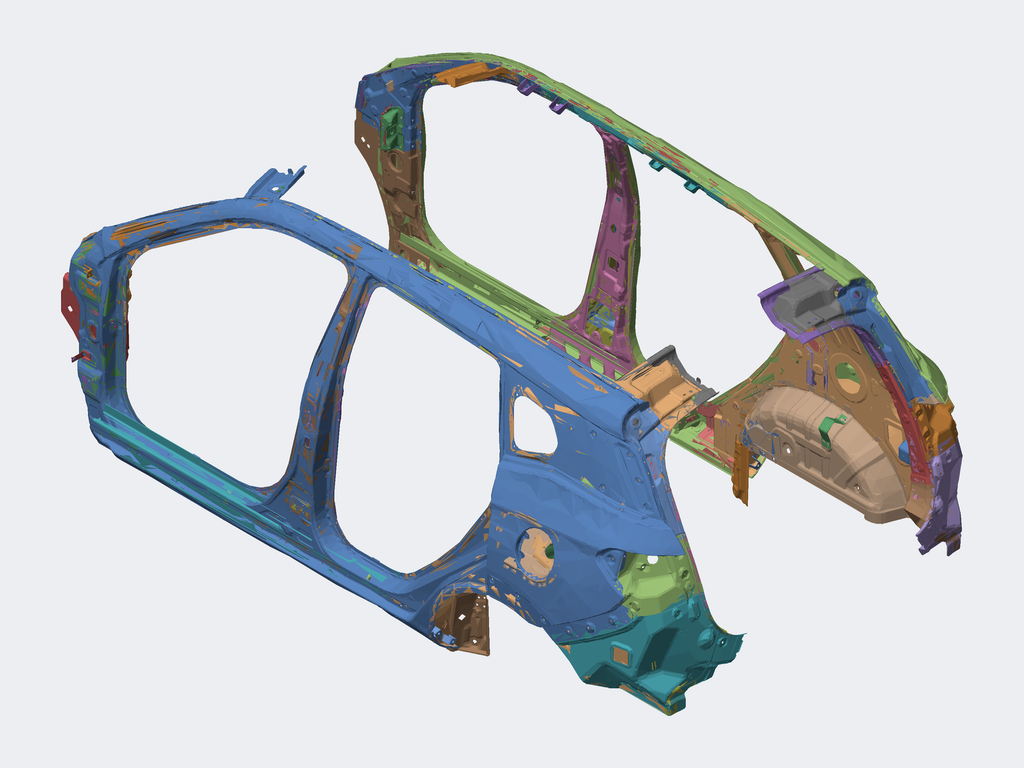Assembly | STEP file | 146 different items | 273 placed
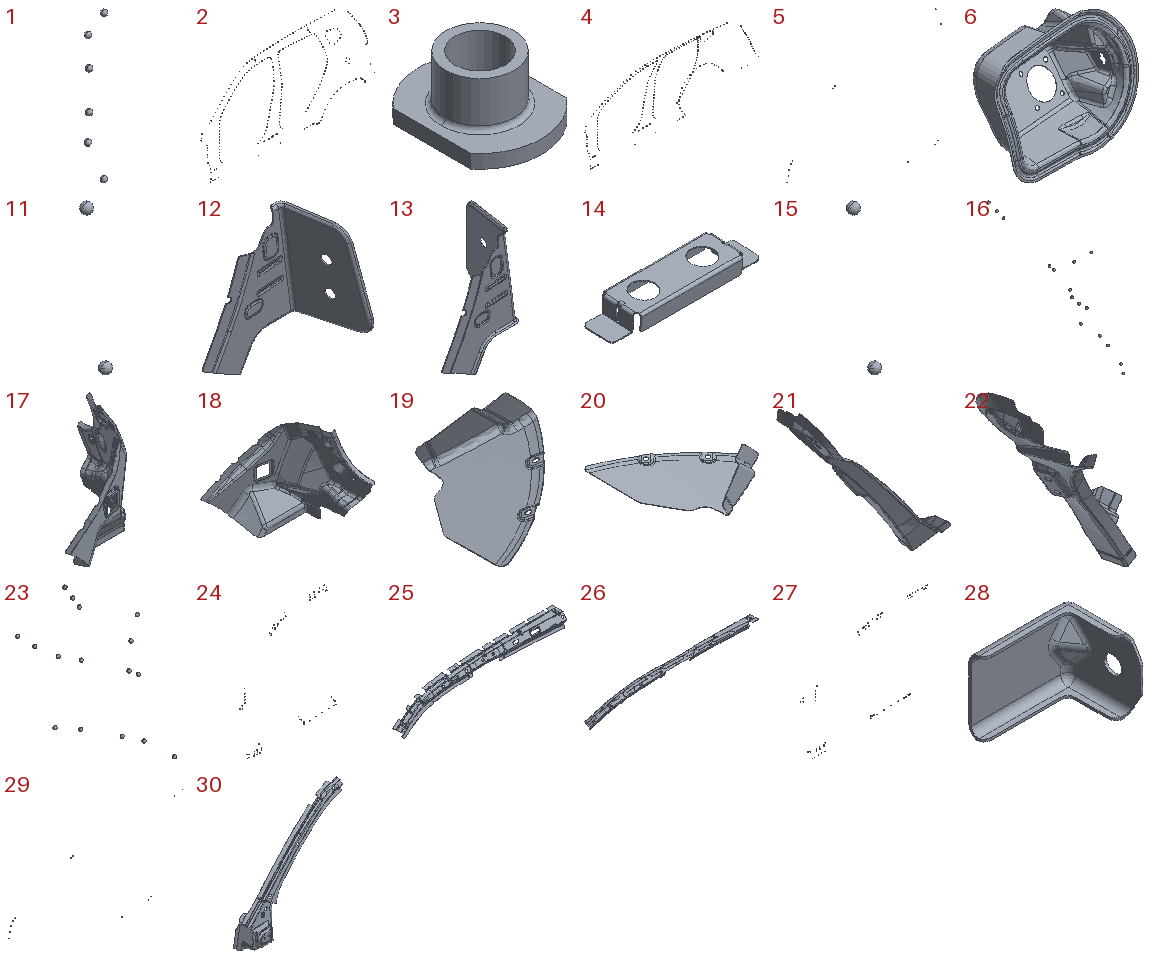Parts list (item | name | quantity | parent item | size | volume):
1 | FN5401370-H | x1 | in FNA5401370 | - | -
2 | FNA5401010-H | x1 | in FNA5401010 | - | -
3 | FNA5401011 | x12 | in FNA5401510, FNA5401520, FNA5401530, FNA5401540, FNA5401830, FNA5401840, FNA5401950, FNA5401960 | 21 x 27 x 13 mm | 2051 mm3
4 | FNA5401020-H | x1 | in FNA5401020 | - | -
5 | FNA5401100-H | x1 | in FNA5401100 | - | -
6 | FNA5401101 | x1 | in FNA5401110 | 305.711 x 153.486 x 230.44 mm | 76829 mm3
7 | FNA5401110-H | x1 | in FNA5401110 | - | -
8 | FNA5401111 | x1 | in FNA5401110 | - | -
9 | FNA5401112 | x1 | in FNA5401120 | - | -
10 | FNA5401120-H | x1 | in FNA5401120 | - | -
11 | FNA5401130-H | x1 | in FNA5401130 | - | -
12 | FNA5401131 | x1 | in FNA5401130 | 126.55 x 90.381 x 162.439 mm | 23457 mm3
13 | FNA5401132 | x1 | in FNA5401140 | 126.55 x 90.381 x 162.439 mm | 23442 mm3
14 | FNA5401133 | x4 | in FNA5401130, FNA5401140, FNA5401250, FNA5401260 | 102.073 x 26.855 x 12.87 mm | 2645 mm3
15 | FNA5401140-H | x1 | in FNA5401140 | - | -
16 | FNA5401150-H | x1 | in FNA5401150 | - | -
17 | FNA5401151 | x1 | in FNA5401150 | 516 x 448.464 x 475.039 mm | 197748 mm3
18 | FNA5401152 | x1 | in FNA5401160 | 516.001 x 448.464 x 475.039 mm | 197648 mm3
19 | FNA5401153 | x1 | in FNA5401150 | 165.89 x 168.782 x 61.393 mm | 13779 mm3
20 | FNA5401154 | x1 | in FNA5401160 | 165.89 x 168.782 x 61.393 mm | 13774 mm3
21 | FNA5401155 | x1 | in FNA5401150 | 332 x 187.997 x 427.512 mm | 56977 mm3
22 | FNA5401156 | x1 | in FNA5401160 | 332 x 187.997 x 427.512 mm | 56978 mm3
23 | FNA5401160-H | x1 | in FNA5401160 | - | -
24 | FNA5401170-H | x1 | in FNA5401170 | - | -
25 | FNA5401171 | x1 | in FNA5401170 | 1257 x 126.52 x 207.673 mm | 214669 mm3
26 | FNA5401172 | x1 | in FNA5401180 | 1257 x 126.52 x 207.673 mm | 214644 mm3
27 | FNA5401180-H | x1 | in FNA5401180 | - | -
28 | FNA5401191 | x2 | in FNA5401190 | 40.165 x 30.291 x 30.011 mm | 2314 mm3
29 | FNA5401200-H | x1 | in FNA5401200 | - | -
30 | FNA5401211 | x1 | in FNA5401210 | 914.927 x 216.551 x 677.274 mm | 215697 mm3
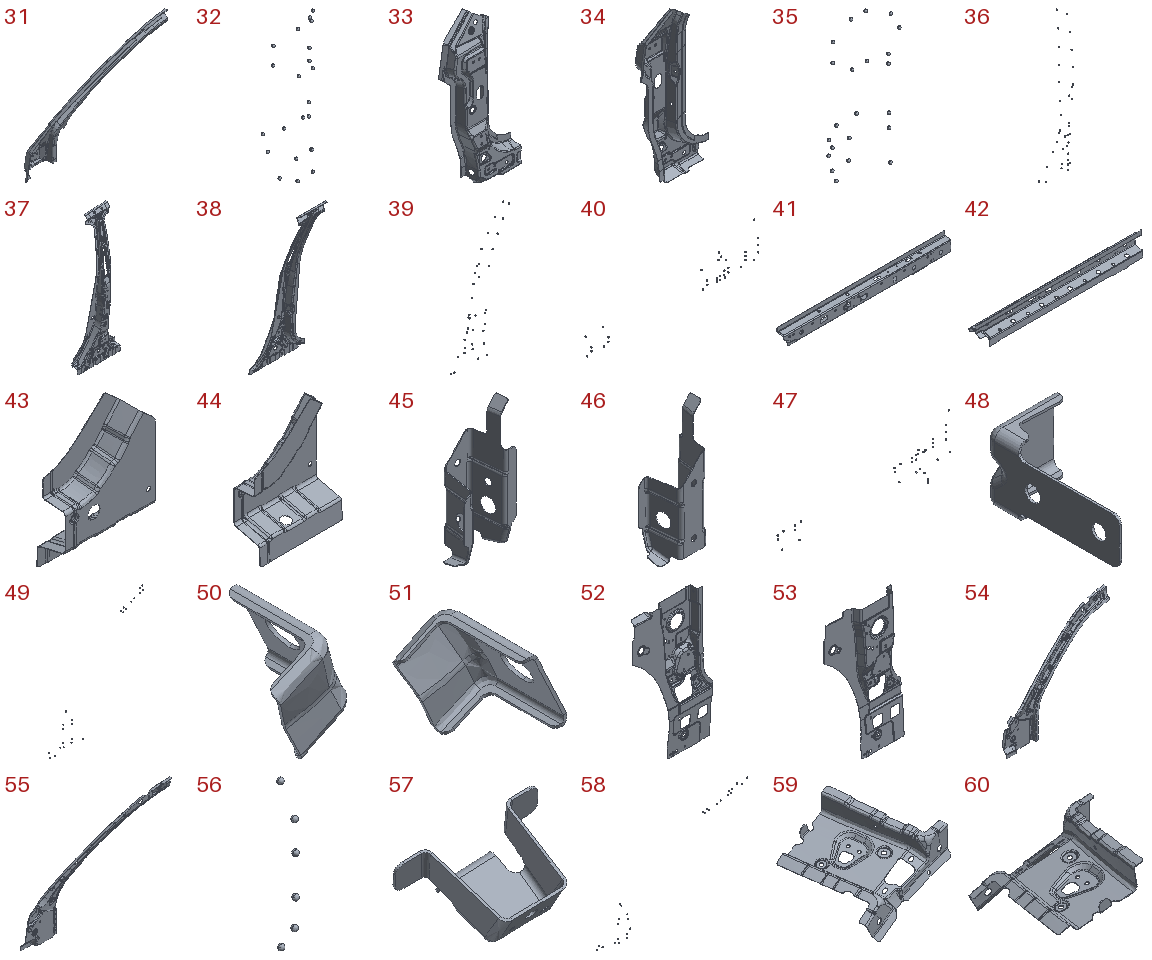31 | FNA5401212 | x1 | in FNA5401220 | 914.927 x 216.551 x 677.274 mm | 214602 mm3
32 | FNA5401230-H | x1 | in FNA5401230 | - | -
33 | FNA5401231 | x1 | in FNA5401230 | 393.159 x 114.364 x 853.043 mm | 316427 mm3
34 | FNA5401232 | x1 | in FNA5401240 | 393.159 x 114.364 x 853.043 mm | 316443 mm3
35 | FNA5401240-H | x1 | in FNA5401240 | - | -
36 | FNA5401250-H | x1 | in FNA5401250 | - | -
37 | FNA5401251 | x1 | in FNA5401250 | 510.856 x 226.55 x 1230 mm | 703654 mm3
38 | FNA5401252 | x1 | in FNA5401260 | 510.856 x 226.55 x 1230 mm | 703226 mm3
39 | FNA5401260-H | x1 | in FNA5401260 | - | -
40 | FNA5401270-H | x1 | in FNA5401270 | - | -
41 | FNA5401271 | x1 | in FNA5401270 | 1459 x 72.45 x 212.137 mm | 599256 mm3
42 | FNA5401272 | x1 | in FNA5401280 | 1459 x 72.45 x 212.137 mm | 599256 mm3
43 | FNA5401273 | x1 | in FNA5401270 | 220.5 x 72.73 x 306.154 mm | 92619 mm3
44 | FNA5401274 | x1 | in FNA5401280 | 220.5 x 72.73 x 306.154 mm | 92619 mm3
45 | FNA5401275 | x1 | in FNA5401270 | 90 x 57.5 x 220.985 mm | 30019 mm3
46 | FNA5401276 | x1 | in FNA5401280 | 90 x 57.5 x 220.985 mm | 30013 mm3
47 | FNA5401280-H | x1 | in FNA5401280 | - | -
48 | FNA5401291 | x2 | in FNA5401290 | 30.161 x 60.798 x 30.791 mm | 2443 mm3
49 | FNA5401300-H | x1 | in FNA5401300 | - | -
50 | FNA5401311 | x1 | in FNA5401300 | 33.614 x 36.273 x 38.59 mm | 2270 mm3
51 | FNA5401321 | x1 | in FNA5401400 | 33.613 x 36.273 x 38.59 mm | 2270 mm3
52 | FNA5401331 | x1 | in FNA5401330 | 367 x 39.355 x 636.857 mm | 124897 mm3
53 | FNA5401332 | x1 | in FNA5401340 | 367 x 39.355 x 636.857 mm | 124786 mm3
54 | FNA5401351 | x1 | in FNA5401350 | 1045 x 172.359 x 753.685 mm | 232138 mm3
55 | FNA5401352 | x1 | in FNA5401360 | 1045 x 172.359 x 753.685 mm | 232159 mm3
56 | FNA5401380-H | x1 | in FNA5401380 | - | -
57 | FNA5401391 | x2 | in FNA5401390 | 86.183 x 71.891 x 52.032 mm | 9472 mm3
58 | FNA5401400-H | x1 | in FNA5401400 | - | -
59 | FNA5401411 | x1 | in FNA5401410 | 243.972 x 240.219 x 155.739 mm | 51999 mm3
60 | FNA5401412 | x1 | in FNA5401420 | 243.972 x 240.219 x 155.739 mm | 52004 mm3
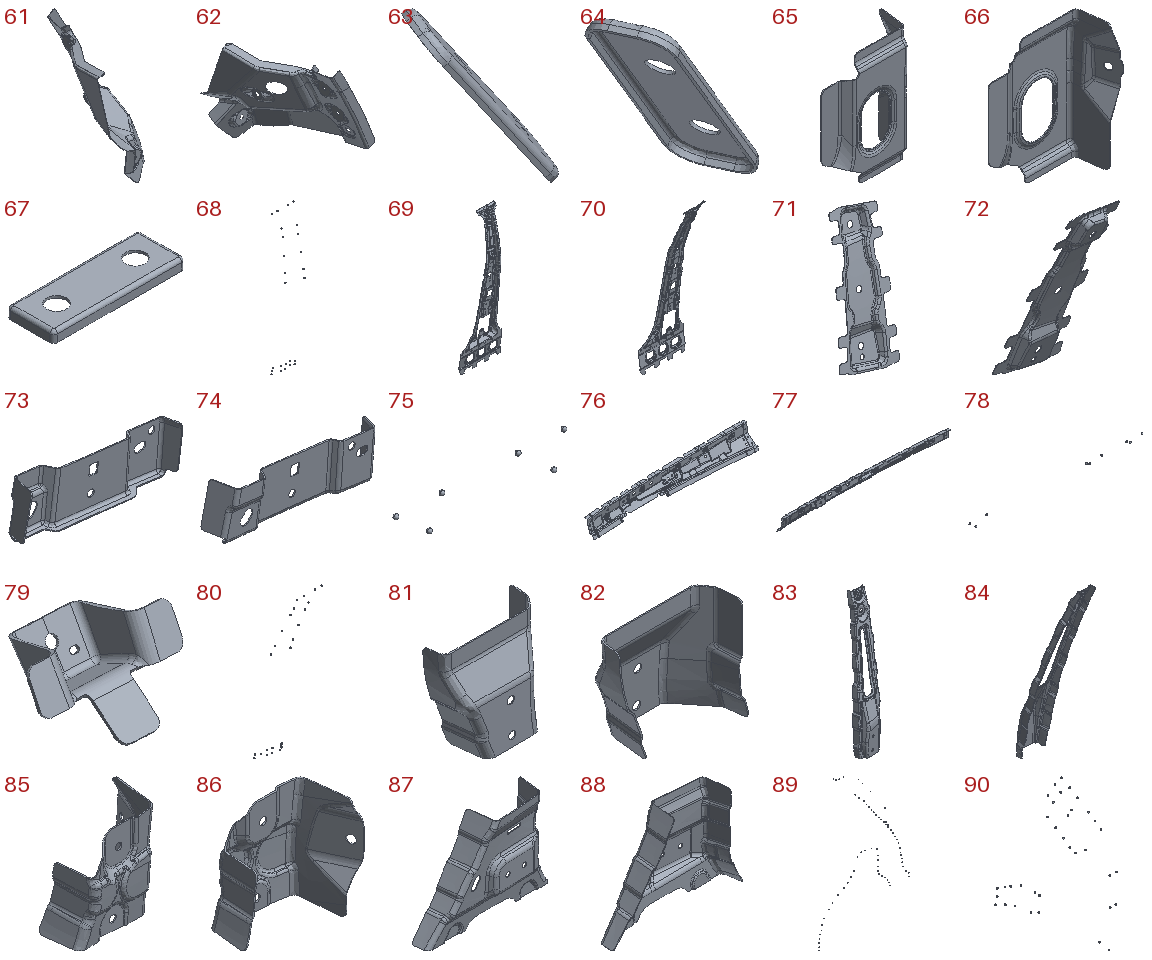61 | FNA5401431 | x1 | in FNA5401430 | 186.295 x 264.478 x 250.717 mm | 73850 mm3
62 | FNA5401432 | x1 | in FNA5401440 | 186.294 x 264.478 x 250.717 mm | 73735 mm3
63 | FNA5401451 | x1 | in FNA5401450 | 62.39 x 39.872 x 86.052 mm | 4191 mm3
64 | FNA5401452 | x1 | in FNA5401460 | 62.39 x 39.872 x 86.052 mm | 4191 mm3
65 | FNA5401471 | x1 | in FNA5401470 | 130.972 x 49.584 x 160 mm | 24899 mm3
66 | FNA5401472 | x1 | in FNA5401480 | 130.972 x 49.584 x 160 mm | 24898 mm3
67 | FNA5401491 | x4 | in FNA5401490 | 67 x 24 x 5.5 mm | 2539 mm3
68 | FNA5401500-H | x1 | in FNA5401500 | - | -
69 | FNA5401511 | x1 | in FNA5401510 | 496.598 x 154.254 x 1271 mm | 355104 mm3
70 | FNA5401512 | x1 | in FNA5401520 | 496.591 x 154.254 x 1271 mm | 354835 mm3
71 | FNA5401531 | x1 | in FNA5401530 | 167.899 x 102.592 x 304.372 mm | 32215 mm3
72 | FNA5401532 | x1 | in FNA5401540 | 167.899 x 102.592 x 304.372 mm | 32208 mm3
73 | FNA5401551 | x1 | in FNA5401550 | 170.503 x 25.651 x 68.139 mm | 12125 mm3
74 | FNA5401552 | x1 | in FNA5401560 | 170.503 x 25.651 x 68.139 mm | 12125 mm3
75 | FNA5401570-H | x1 | in FNA5401570 | - | -
76 | FNA5401571 | x1 | in FNA5401570 | 935.734 x 89.628 x 121.004 mm | 119563 mm3
77 | FNA5401572 | x1 | in FNA5401580 | 935.734 x 89.628 x 121.004 mm | 119341 mm3
78 | FNA5401580-H | x1 | in FNA5401580 | - | -
79 | FNA5401591 | x4 | in FNA5401590 | 84.51 x 63.094 x 41.379 mm | 7895 mm3
80 | FNA5401600-H | x1 | in FNA5401600 | - | -
81 | FNA5401611 | x1 | in FNA5401610 | 135.06 x 63.583 x 123.582 mm | 33584 mm3
82 | FNA5401612 | x1 | in FNA5401620 | 135.06 x 63.583 x 123.582 mm | 33580 mm3
83 | FNA5401631 | x1 | in FNA5401630 | 144.102 x 149.837 x 505.997 mm | 84587 mm3
84 | FNA5401632 | x1 | in FNA5401640 | 144.102 x 149.837 x 505.997 mm | 84587 mm3
85 | FNA5401651 | x1 | in FNA5401650 | 112.986 x 67.931 x 109.011 mm | 25082 mm3
86 | FNA5401652 | x1 | in FNA5401660 | 112.986 x 67.931 x 109.011 mm | 25082 mm3
87 | FNA5401671 | x1 | in FNA5401670 | 254.233 x 59.892 x 176.91 mm | 64853 mm3
88 | FNA5401672 | x1 | in FNA5401680 | 254.233 x 59.892 x 176.91 mm | 65515 mm3
89 | FNA5401700-H | x1 | in FNA5401700 | - | -
90 | FNA5401710-H | x1 | in FNA5401710 | - | -
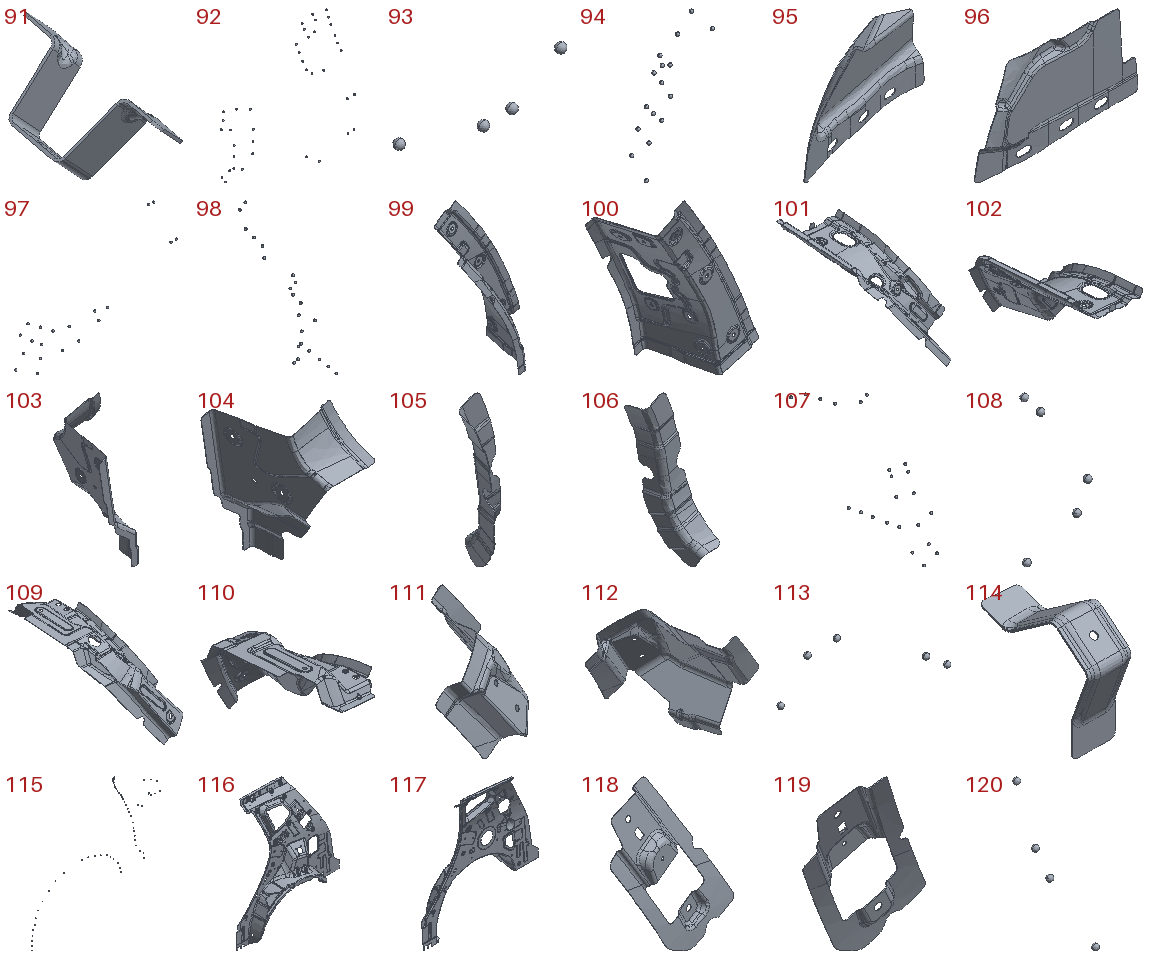91 | FNA5401711 | x2 | in FNA5401710, FNA5401720 | 34.513 x 61.465 x 33.785 mm | 1594 mm3
92 | FNA5401720-H | x1 | in FNA5401720 | - | -
93 | FNA5401730-H | x1 | in FNA5401835 | - | -
94 | FNA5401730-H_1 | x1 | in FNA5401730 | - | -
95 | FNA5401731 | x1 | in FNA5401730 | 225.797 x 47.255 x 140.75 mm | 31228 mm3
96 | FNA5401732 | x1 | in FNA5401740 | 225.882 x 22.076 x 141.359 mm | 28892 mm3
97 | FNA5401740-H | x1 | in FNA5401740 | - | -
98 | FNA5401750-H | x1 | in FNA5401750 | - | -
99 | FNA5401751 | x1 | in FNA5401310 | 337.448 x 183.804 x 466.44 mm | 116548 mm3
100 | FNA5401752 | x1 | in FNA5401320 | 337.448 x 183.804 x 466.44 mm | 116602 mm3
101 | FNA5401753 | x1 | in FNA5401750 | 326.803 x 462.989 x 355.554 mm | 121540 mm3
102 | FNA5401754 | x1 | in FNA5401760 | 326.803 x 462.989 x 355.554 mm | 121571 mm3
103 | FNA5401755 | x1 | in FNA5401750 | 204.272 x 236.4 x 380.596 mm | 84928 mm3
104 | FNA5401756 | x1 | in FNA5401760 | 204.272 x 236.4 x 380.596 mm | 84929 mm3
105 | FNA5401757 | x1 | in FNA5401750 | 100.489 x 85.531 x 281.294 mm | 19458 mm3
106 | FNA5401758 | x1 | in FNA5401760 | 100.489 x 85.531 x 281.294 mm | 19458 mm3
107 | FNA5401760-H | x1 | in FNA5401760 | - | -
108 | FNA5401770-H | x1 | in FNA5401770 | - | -
109 | FNA5401771 | x1 | in FNA5401770 | 311.119 x 450.581 x 343.825 mm | 154298 mm3
110 | FNA5401772 | x1 | in FNA5401780 | 311.119 x 450.58 x 343.825 mm | 154252 mm3
111 | FNA5401773 | x1 | in FNA5401770 | 196.776 x 165.218 x 196.033 mm | 33509 mm3
112 | FNA5401774 | x1 | in FNA5401780 | 196.776 x 165.218 x 196.033 mm | 33509 mm3
113 | FNA5401780-H | x1 | in FNA5401780 | - | -
114 | FNA5401791 | x1 | in FNA5401790 | 42.218 x 112.188 x 109.748 mm | 13572 mm3
115 | FNA5401800-H | x1 | in FNA5401800 | - | -
116 | FNA5401811 | x1 | in FNA5401810 | 1194 x 381.776 x 1328 mm | 682767 mm3
117 | FNA5401812 | x1 | in FNA5401820 | 1194 x 381.773 x 1328 mm | 686695 mm3
118 | FNA5401831 | x1 | in FNA5401830 | 269.629 x 81.435 x 345.025 mm | 52905 mm3
119 | FNA5401832 | x1 | in FNA5401840 | 269.629 x 81.435 x 345.025 mm | 52905 mm3
120 | FNA5401836-H | x1 | in FNA5401836 | - | -
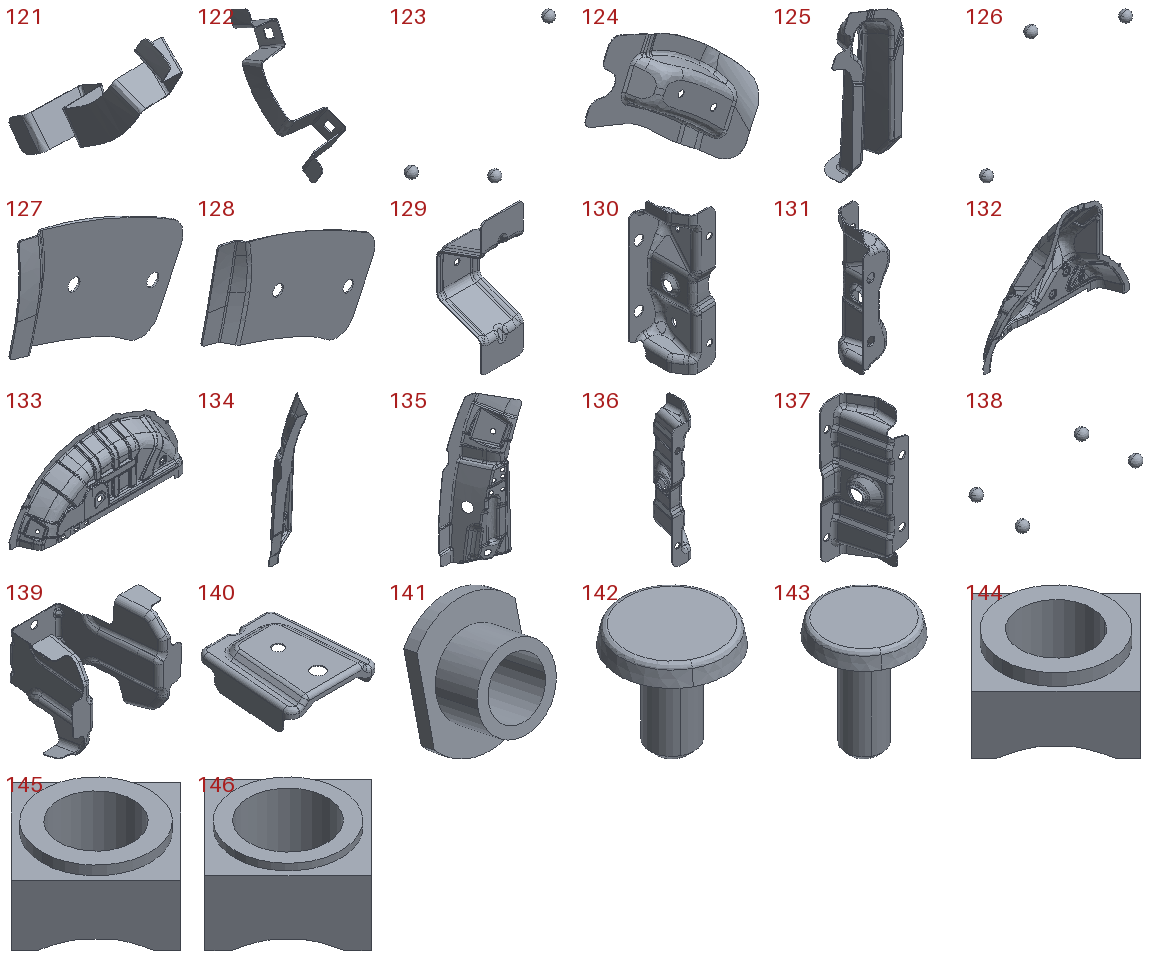121 | FNA5401837 | x1 | in FNA5401835 | 44.202 x 118.87 x 119.505 mm | 6315 mm3
122 | FNA5401838 | x1 | in FNA5401836 | 44.202 x 118.87 x 119.505 mm | 6315 mm3
123 | FNA5401850-H | x1 | in FNA5401850 | - | -
124 | FNA5401851 | x1 | in FNA5401850 | 189.152 x 47.956 x 178.015 mm | 18533 mm3
125 | FNA5401852 | x1 | in FNA5401860 | 144.073 x 78.491 x 318.118 mm | 43750 mm3
126 | FNA5401860-H | x1 | in FNA5401860 | - | -
127 | FNA5401871 | x1 | in FNA5401870 | 183.449 x 12.361 x 148.782 mm | 24633 mm3
128 | FNA5401872 | x1 | in FNA5401880 | 183.448 x 12.361 x 148.783 mm | 24633 mm3
129 | FNA5401891 | x2 | in FNA5401890 | 50 x 55.964 x 158.896 mm | 17278 mm3
130 | FNA5401911 | x1 | in FNA5401910 | 52.06 x 60.819 x 178.002 mm | 29929 mm3
131 | FNA5401912 | x1 | in FNA5401920 | 52.06 x 60.819 x 178.002 mm | 29907 mm3
132 | FNA5401931 | x1 | in FNA5401930 | 852.046 x 163.068 x 589.293 mm | 275736 mm3
133 | FNA5401932 | x1 | in FNA5401740 | 852.046 x 115.257 x 334.468 mm | 191833 mm3
134 | FNA5401951 | x1 | in FNA5401950 | 173.275 x 92.989 x 412.618 mm | 89975 mm3
135 | FNA5401952 | x1 | in FNA5401960 | 172.44 x 97.142 x 412.618 mm | 89777 mm3
136 | FNA5401971 | x1 | in FNA5401970 | 55.243 x 59.367 x 177.004 mm | 26193 mm3
137 | FNA5401972 | x1 | in FNA5401980 | 55.243 x 59.367 x 177.004 mm | 26149 mm3
138 | FNA5401990-H | x4 | in FNA5401990 | - | -
139 | FNA5401991 | x4 | in FNA5401990 | 121.896 x 103.862 x 100.696 mm | 16854 mm3
140 | FNA5401992 | x4 | in FNA5401990 | 66.933 x 77 x 22.144 mm | 6040 mm3
141 | FNA6101013 | x8 | in FNA5401490 | 14.049 x 11.577 x 17.992 mm | 641.835 mm3
142 | Q1980612 | x2 | in FNA5401290 | 14.5 x 14.5 x 14.5 mm | 715.577 mm3
143 | Q1980616 | x3 | in FNA5401930 | 14.5 x 14.5 x 18.5 mm | 828.674 mm3
144 | Q37106 | x44 | in FNA5401190, FNA5401310, FNA5401320, FNA5401330, FNA5401340, FNA5401390, FNA5401410, FNA5401420, FNA5401510, FNA5401520, FNA5401550, FNA5401560, FNA5401590, FNA5401790, FNA5401810, FNA5401820, FNA5401830, FNA5401840, FNA5401890, FNA5401930 | 14.142 x 14.142 x 5.9 mm | 331.042 mm3
145 | Q37108 | x38 | in FNA5401210, FNA5401220, FNA5401330, FNA5401340, FNA5401350, FNA5401360, FNA5401450, FNA5401460, FNA5401470, FNA5401480, FNA5401610, FNA5401620, FNA5401630, FNA5401640, FNA5401650, FNA5401660, FNA5401670, FNA5401680, FNA5401910, FNA5401920, FNA5401970, FNA5401980 | 18.385 x 18.385 x 7.6 mm | 729.18 mm3
146 | Q37110 | x4 | in FNA5401870, FNA5401880 | 21.213 x 21.213 x 9.167 mm | 1120 mm3